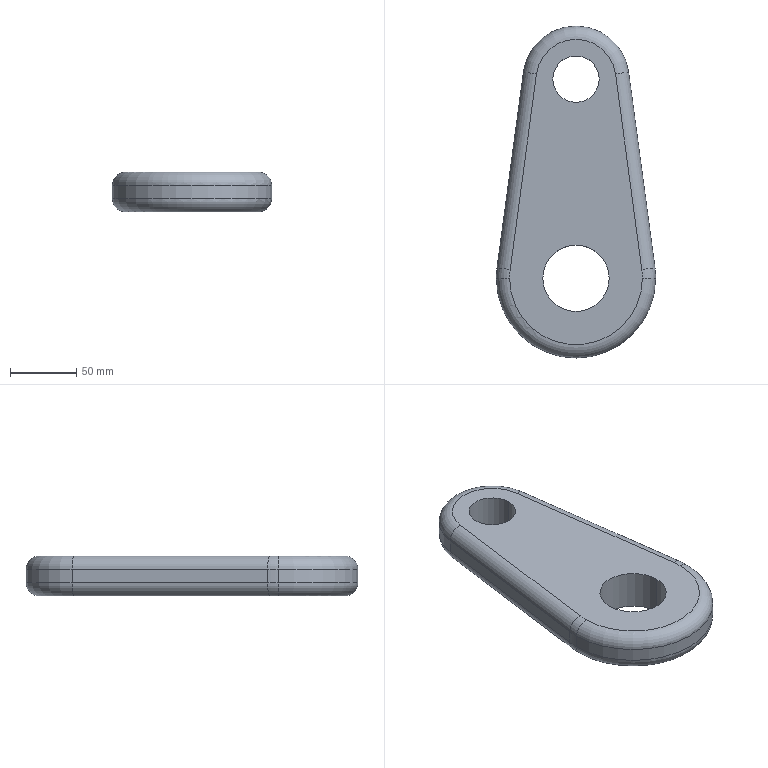Part | SolidWorks | features HoleWzd 2, Extrusion 1, Fillet 1 | 1 solid | 24 faces | box 120 x 250 x 30 mm | volume 585410 mm3 | cylinder 12 | torus 8 | plane 4 | commonest cylinder face diameters 20 x4 120 x3 35 x2 50 x2 80 x1
STEP:
#1=CARTESIAN_POINT('',(-50.,0.,0.));
#2=VERTEX_POINT('',#1);
#3=CARTESIAN_POINT('',(-49.554,6.667,0.));
#4=VERTEX_POINT('',#3);
#5=CARTESIAN_POINT('',(0.,0.,0.));
#6=DIRECTION('',(0.,0.,-1.));
#7=DIRECTION('',(1.,0.,0.));
#8=AXIS2_PLACEMENT_3D('',#5,#6,#7);
#9=CIRCLE('',#8,50.);
#10=EDGE_CURVE('',#2,#4,#9,.T.);
#11=ORIENTED_EDGE('',*,*,#10,.F.);
#12=CARTESIAN_POINT('',(-60.,0.,10.));
#13=VERTEX_POINT('',#12);
#14=CARTESIAN_POINT('',(-50.,0.,10.));
#15=DIRECTION('',(0.,1.,0.));
#16=DIRECTION('',(-1.,0.,0.));
#17=AXIS2_PLACEMENT_3D('',#14,#15,#16);
#18=CIRCLE('',#17,10.);
#19=EDGE_CURVE('',#2,#13,#18,.T.);
#20=ORIENTED_EDGE('',*,*,#19,.T.);
#21=CARTESIAN_POINT('',(-59.464,8.,10.));
#22=VERTEX_POINT('',#21);
#23=CARTESIAN_POINT('',(0.,0.,10.));
#24=DIRECTION('',(0.,0.,1.));
#25=DIRECTION('',(1.,0.,0.));
#26=AXIS2_PLACEMENT_3D('',#23,#24,#25);
#27=CIRCLE('',#26,60.);
#28=EDGE_CURVE('',#22,#13,#27,.T.);
#29=ORIENTED_EDGE('',*,*,#28,.F.);
#30=CARTESIAN_POINT('',(-49.554,6.667,10.));
#31=DIRECTION('',(-0.1333,-0.9911,0.));
#32=DIRECTION('',(0.9911,-0.1333,0.));
#33=AXIS2_PLACEMENT_3D('',#30,#31,#32);
#34=CIRCLE('',#33,10.);
#35=EDGE_CURVE('',#22,#4,#34,.T.);
#36=ORIENTED_EDGE('',*,*,#35,.T.);
#37=EDGE_LOOP('',(#11,#20,#29,#36));
#38=FACE_OUTER_BOUND('',#37,.T.);
#39=CARTESIAN_POINT('',(0.,0.,10.));
#40=DIRECTION('',(0.,0.,1.));
#41=DIRECTION('',(1.,0.,0.));
#42=AXIS2_PLACEMENT_3D('',#39,#40,#41);
#43=TOROIDAL_SURFACE('',#42,50.,10.);
#44=ADVANCED_FACE('',(#38),#43,.T.);
#45=ORIENTED_EDGE('',*,*,#19,.F.);
#46=CARTESIAN_POINT('',(50.,0.,0.));
#47=VERTEX_POINT('',#46);
#48=CARTESIAN_POINT('',(0.,0.,0.));
#49=DIRECTION('',(0.,0.,-1.));
#50=DIRECTION('',(1.,0.,0.));
#51=AXIS2_PLACEMENT_3D('',#48,#49,#50);
#52=CIRCLE('',#51,50.);
#53=EDGE_CURVE('',#47,#2,#52,.T.);
#54=ORIENTED_EDGE('',*,*,#53,.F.);
#55=CARTESIAN_POINT('',(60.,0.,10.));
#56=VERTEX_POINT('',#55);
#57=CARTESIAN_POINT('',(50.,0.,10.));
#58=DIRECTION('',(0.,-1.,0.));
#59=DIRECTION('',(0.,0.,-1.));
#60=AXIS2_PLACEMENT_3D('',#57,#58,#59);
#61=CIRCLE('',#60,10.);
#62=EDGE_CURVE('',#47,#56,#61,.T.);
#63=ORIENTED_EDGE('',*,*,#62,.T.);
#64=CARTESIAN_POINT('',(0.,0.,10.));
#65=DIRECTION('',(0.,0.,1.));
#66=DIRECTION('',(1.,0.,0.));
#67=AXIS2_PLACEMENT_3D('',#64,#65,#66);
#68=CIRCLE('',#67,60.);
#69=EDGE_CURVE('',#13,#56,#68,.T.);
#70=ORIENTED_EDGE('',*,*,#69,.F.);
#71=EDGE_LOOP('',(#45,#54,#63,#70));
#72=FACE_OUTER_BOUND('',#71,.T.);
#73=CARTESIAN_POINT('',(0.,0.,10.));
#74=DIRECTION('',(0.,0.,1.));
#75=DIRECTION('',(1.,0.,0.));
#76=AXIS2_PLACEMENT_3D('',#73,#74,#75);
#77=TOROIDAL_SURFACE('',#76,50.,10.);
#78=ADVANCED_FACE('',(#72),#77,.T.);
#79=CARTESIAN_POINT('',(-60.,0.,20.));
#80=VERTEX_POINT('',#79);
#81=CARTESIAN_POINT('',(-59.464,8.,20.));
#82=VERTEX_POINT('',#81);
#83=CARTESIAN_POINT('',(0.,0.,20.));
#84=DIRECTION('',(0.,0.,-1.));
#85=DIRECTION('',(1.,0.,0.));
#86=AXIS2_PLACEMENT_3D('',#83,#84,#85);
#87=CIRCLE('',#86,60.);
#88=EDGE_CURVE('',#80,#82,#87,.T.);
#89=ORIENTED_EDGE('',*,*,#88,.F.);
#90=CARTESIAN_POINT('',(-50.,0.,30.));
#91=VERTEX_POINT('',#90);
#92=CARTESIAN_POINT('',(-50.,0.,20.));
#93=DIRECTION('',(0.,1.,0.));
#94=DIRECTION('',(-1.,0.,0.));
#95=AXIS2_PLACEMENT_3D('',#92,#93,#94);
#96=CIRCLE('',#95,10.);
#97=EDGE_CURVE('',#80,#91,#96,.T.);
#98=ORIENTED_EDGE('',*,*,#97,.T.);
#99=CARTESIAN_POINT('',(-49.554,6.667,30.));
#100=VERTEX_POINT('',#99);
#101=CARTESIAN_POINT('',(0.,0.,30.));
#102=DIRECTION('',(0.,0.,1.));
#103=DIRECTION('',(1.,0.,0.));
#104=AXIS2_PLACEMENT_3D('',#101,#102,#103);
#105=CIRCLE('',#104,50.);
#106=EDGE_CURVE('',#100,#91,#105,.T.);
#107=ORIENTED_EDGE('',*,*,#106,.F.);
#108=CARTESIAN_POINT('',(-49.554,6.667,20.));
#109=DIRECTION('',(0.1333,0.9911,0.));
#110=DIRECTION('',(-0.9911,0.1333,0.));
#111=AXIS2_PLACEMENT_3D('',#108,#109,#110);
#112=CIRCLE('',#111,10.);
#113=EDGE_CURVE('',#82,#100,#112,.T.);
#114=ORIENTED_EDGE('',*,*,#113,.F.);
#115=EDGE_LOOP('',(#89,#98,#107,#114));
#116=FACE_OUTER_BOUND('',#115,.T.);
#117=CARTESIAN_POINT('',(0.,0.,20.));
#118=DIRECTION('',(0.,0.,1.));
#119=DIRECTION('',(1.,0.,0.));
#120=AXIS2_PLACEMENT_3D('',#117,#118,#119);
#121=TOROIDAL_SURFACE('',#120,50.,10.);
#122=ADVANCED_FACE('',(#116),#121,.T.);
#123=ORIENTED_EDGE('',*,*,#97,.F.);
#124=CARTESIAN_POINT('',(60.,0.,20.));
#125=VERTEX_POINT('',#124);
#126=CARTESIAN_POINT('',(0.,0.,20.));
#127=DIRECTION('',(0.,0.,-1.));
#128=DIRECTION('',(1.,0.,0.));
#129=AXIS2_PLACEMENT_3D('',#126,#127,#128);
#130=CIRCLE('',#129,60.);
#131=EDGE_CURVE('',#125,#80,#130,.T.);
#132=ORIENTED_EDGE('',*,*,#131,.F.);
#133=CARTESIAN_POINT('',(50.,0.,30.));
#134=VERTEX_POINT('',#133);
#135=CARTESIAN_POINT('',(50.,0.,20.));
#136=DIRECTION('',(0.,-1.,0.));
#137=DIRECTION('',(0.,0.,-1.));
#138=AXIS2_PLACEMENT_3D('',#135,#136,#137);
#139=CIRCLE('',#138,10.);
#140=EDGE_CURVE('',#125,#134,#139,.T.);
#141=ORIENTED_EDGE('',*,*,#140,.T.);
#142=CARTESIAN_POINT('',(0.,0.,30.));
#143=DIRECTION('',(0.,0.,1.));
#144=DIRECTION('',(1.,0.,0.));
#145=AXIS2_PLACEMENT_3D('',#142,#143,#144);
#146=CIRCLE('',#145,50.);
#147=EDGE_CURVE('',#91,#134,#146,.T.);
#148=ORIENTED_EDGE('',*,*,#147,.F.);
#149=EDGE_LOOP('',(#123,#132,#141,#148));
#150=FACE_OUTER_BOUND('',#149,.T.);
#151=CARTESIAN_POINT('',(0.,0.,20.));
#152=DIRECTION('',(0.,0.,1.));
#153=DIRECTION('',(1.,0.,0.));
#154=AXIS2_PLACEMENT_3D('',#151,#152,#153);
#155=TOROIDAL_SURFACE('',#154,50.,10.);
#156=ADVANCED_FACE('',(#150),#155,.T.);
#157=CARTESIAN_POINT('',(25.,0.,30.));
#158=VERTEX_POINT('',#157);
#159=CARTESIAN_POINT('',(-25.,0.,30.));
#160=VERTEX_POINT('',#159);
#161=CARTESIAN_POINT('',(0.,0.,30.));
#162=DIRECTION('',(0.,0.,-1.));
#163=DIRECTION('',(-1.,0.,0.));
#164=AXIS2_PLACEMENT_3D('',#161,#162,#163);
#165=CIRCLE('',#164,25.);
#166=EDGE_CURVE('',#158,#160,#165,.T.);
#167=ORIENTED_EDGE('',*,*,#166,.F.);
#168=CARTESIAN_POINT('',(25.,0.,0.));
#169=VERTEX_POINT('',#168);
#170=CARTESIAN_POINT('',(25.,0.,0.));
#171=DIRECTION('',(0.,0.,-1.));
#172=VECTOR('',#171,1000.);
#173=LINE('',#170,#172);
#174=EDGE_CURVE('',#158,#169,#173,.T.);
#175=ORIENTED_EDGE('',*,*,#174,.T.);
#176=CARTESIAN_POINT('',(-25.,0.,0.));
#177=VERTEX_POINT('',#176);
#178=CARTESIAN_POINT('',(0.,0.,0.));
#179=DIRECTION('',(0.,0.,-1.));
#180=DIRECTION('',(-1.,0.,0.));
#181=AXIS2_PLACEMENT_3D('',#178,#179,#180);
#182=CIRCLE('',#181,25.);
#183=EDGE_CURVE('',#169,#177,#182,.T.);
#184=ORIENTED_EDGE('',*,*,#183,.T.);
#185=CARTESIAN_POINT('',(-25.,0.,0.));
#186=DIRECTION('',(0.,0.,-1.));
#187=VECTOR('',#186,1000.);
#188=LINE('',#185,#187);
#189=EDGE_CURVE('',#160,#177,#188,.T.);
#190=ORIENTED_EDGE('',*,*,#189,.F.);
#191=EDGE_LOOP('',(#167,#175,#184,#190));
#192=FACE_OUTER_BOUND('',#191,.T.);
#193=CARTESIAN_POINT('',(0.,0.,0.));
#194=DIRECTION('',(0.,0.,-1.));
#195=DIRECTION('',(-1.,0.,0.));
#196=AXIS2_PLACEMENT_3D('',#193,#194,#195);
#197=CYLINDRICAL_SURFACE('',#196,25.);
#198=ADVANCED_FACE('',(#192),#197,.F.);
#199=CARTESIAN_POINT('',(17.5,150.,30.));
#200=VERTEX_POINT('',#199);
#201=CARTESIAN_POINT('',(-17.5,150.,30.));
#202=VERTEX_POINT('',#201);
#203=CARTESIAN_POINT('',(0.,150.,30.));
#204=DIRECTION('',(0.,0.,-1.));
#205=DIRECTION('',(-1.,0.,0.));
#206=AXIS2_PLACEMENT_3D('',#203,#204,#205);
#207=CIRCLE('',#206,17.5);
#208=EDGE_CURVE('',#200,#202,#207,.T.);
#209=ORIENTED_EDGE('',*,*,#208,.F.);
#210=CARTESIAN_POINT('',(17.5,150.,0.));
#211=VERTEX_POINT('',#210);
#212=CARTESIAN_POINT('',(17.5,150.,0.));
#213=DIRECTION('',(0.,0.,-1.));
#214=VECTOR('',#213,1000.);
#215=LINE('',#212,#214);
#216=EDGE_CURVE('',#200,#211,#215,.T.);
#217=ORIENTED_EDGE('',*,*,#216,.T.);
#218=CARTESIAN_POINT('',(-17.5,150.,0.));
#219=VERTEX_POINT('',#218);
#220=CARTESIAN_POINT('',(0.,150.,0.));
#221=DIRECTION('',(0.,0.,-1.));
#222=DIRECTION('',(-1.,0.,0.));
#223=AXIS2_PLACEMENT_3D('',#220,#221,#222);
#224=CIRCLE('',#223,17.5);
#225=EDGE_CURVE('',#211,#219,#224,.T.);
#226=ORIENTED_EDGE('',*,*,#225,.T.);
#227=CARTESIAN_POINT('',(-17.5,150.,0.));
#228=DIRECTION('',(0.,0.,-1.));
#229=VECTOR('',#228,1000.);
#230=LINE('',#227,#229);
#231=EDGE_CURVE('',#202,#219,#230,.T.);
#232=ORIENTED_EDGE('',*,*,#231,.F.);
#233=EDGE_LOOP('',(#209,#217,#226,#232));
#234=FACE_OUTER_BOUND('',#233,.T.);
#235=CARTESIAN_POINT('',(0.,150.,0.));
#236=DIRECTION('',(0.,0.,-1.));
#237=DIRECTION('',(-1.,0.,0.));
#238=AXIS2_PLACEMENT_3D('',#235,#236,#237);
#239=CYLINDRICAL_SURFACE('',#238,17.5);
#240=ADVANCED_FACE('',(#234),#239,.F.);
#241=ORIENTED_EDGE('',*,*,#28,.T.);
#242=CARTESIAN_POINT('',(-60.,0.,0.));
#243=DIRECTION('',(0.,0.,1.));
#244=VECTOR('',#243,1000.);
#245=LINE('',#242,#244);
#246=EDGE_CURVE('',#13,#80,#245,.T.);
#247=ORIENTED_EDGE('',*,*,#246,.T.);
#248=ORIENTED_EDGE('',*,*,#88,.T.);
#249=CARTESIAN_POINT('',(-59.464,8.,0.));
#250=DIRECTION('',(0.,0.,1.));
#251=VECTOR('',#250,1000.);
#252=LINE('',#249,#251);
#253=EDGE_CURVE('',#22,#82,#252,.T.);
#254=ORIENTED_EDGE('',*,*,#253,.F.);
#255=EDGE_LOOP('',(#241,#247,#248,#254));
#256=FACE_OUTER_BOUND('',#255,.T.);
#257=CARTESIAN_POINT('',(0.,0.,0.));
#258=DIRECTION('',(0.,0.,1.));
#259=DIRECTION('',(1.,0.,0.));
#260=AXIS2_PLACEMENT_3D('',#257,#258,#259);
#261=CYLINDRICAL_SURFACE('',#260,60.);
#262=ADVANCED_FACE('',(#256),#261,.T.);
#263=ORIENTED_EDGE('',*,*,#246,.F.);
#264=ORIENTED_EDGE('',*,*,#69,.T.);
#265=CARTESIAN_POINT('',(60.,0.,0.));
#266=DIRECTION('',(0.,0.,1.));
#267=VECTOR('',#266,1000.);
#268=LINE('',#265,#267);
#269=EDGE_CURVE('',#56,#125,#268,.T.);
#270=ORIENTED_EDGE('',*,*,#269,.T.);
#271=ORIENTED_EDGE('',*,*,#131,.T.);
#272=EDGE_LOOP('',(#263,#264,#270,#271));
#273=FACE_OUTER_BOUND('',#272,.T.);
#274=CARTESIAN_POINT('',(0.,0.,0.));
#275=DIRECTION('',(0.,0.,1.));
#276=DIRECTION('',(1.,0.,0.));
#277=AXIS2_PLACEMENT_3D('',#274,#275,#276);
#278=CYLINDRICAL_SURFACE('',#277,60.);
#279=ADVANCED_FACE('',(#273),#278,.T.);
#280=ORIENTED_EDGE('',*,*,#269,.F.);
#281=CARTESIAN_POINT('',(59.464,8.,10.));
#282=VERTEX_POINT('',#281);
#283=CARTESIAN_POINT('',(0.,0.,10.));
#284=DIRECTION('',(0.,0.,1.));
#285=DIRECTION('',(1.,0.,0.));
#286=AXIS2_PLACEMENT_3D('',#283,#284,#285);
#287=CIRCLE('',#286,60.);
#288=EDGE_CURVE('',#56,#282,#287,.T.);
#289=ORIENTED_EDGE('',*,*,#288,.T.);
#290=CARTESIAN_POINT('',(59.464,8.,20.));
#291=VERTEX_POINT('',#290);
#292=CARTESIAN_POINT('',(59.464,8.,0.));
#293=DIRECTION('',(0.,0.,1.));
#294=VECTOR('',#293,1000.);
#295=LINE('',#292,#294);
#296=EDGE_CURVE('',#282,#291,#295,.T.);
#297=ORIENTED_EDGE('',*,*,#296,.T.);
#298=CARTESIAN_POINT('',(0.,0.,20.));
#299=DIRECTION('',(0.,0.,-1.));
#300=DIRECTION('',(1.,0.,0.));
#301=AXIS2_PLACEMENT_3D('',#298,#299,#300);
#302=CIRCLE('',#301,60.);
#303=EDGE_CURVE('',#291,#125,#302,.T.);
#304=ORIENTED_EDGE('',*,*,#303,.T.);
#305=EDGE_LOOP('',(#280,#289,#297,#304));
#306=FACE_OUTER_BOUND('',#305,.T.);
#307=CARTESIAN_POINT('',(0.,0.,0.));
#308=DIRECTION('',(0.,0.,1.));
#309=DIRECTION('',(1.,0.,0.));
#310=AXIS2_PLACEMENT_3D('',#307,#308,#309);
#311=CYLINDRICAL_SURFACE('',#310,60.);
#312=ADVANCED_FACE('',(#306),#311,.T.);
#313=ORIENTED_EDGE('',*,*,#253,.T.);
#314=CARTESIAN_POINT('',(-39.643,155.333,20.));
#315=VERTEX_POINT('',#314);
#316=CARTESIAN_POINT('',(-39.643,155.333,20.));
#317=DIRECTION('',(0.1333,0.9911,0.));
#318=VECTOR('',#317,1000.);
#319=LINE('',#316,#318);
#320=EDGE_CURVE('',#82,#315,#319,.T.);
#321=ORIENTED_EDGE('',*,*,#320,.T.);
#322=CARTESIAN_POINT('',(-39.643,155.333,10.));
#323=VERTEX_POINT('',#322);
#324=CARTESIAN_POINT('',(-39.643,155.333,0.));
#325=DIRECTION('',(0.,0.,1.));
#326=VECTOR('',#325,1000.);
#327=LINE('',#324,#326);
#328=EDGE_CURVE('',#323,#315,#327,.T.);
#329=ORIENTED_EDGE('',*,*,#328,.F.);
#330=CARTESIAN_POINT('',(-59.464,8.,10.));
#331=DIRECTION('',(-0.1333,-0.9911,0.));
#332=VECTOR('',#331,1000.);
#333=LINE('',#330,#332);
#334=EDGE_CURVE('',#323,#22,#333,.T.);
#335=ORIENTED_EDGE('',*,*,#334,.T.);
#336=EDGE_LOOP('',(#313,#321,#329,#335));
#337=FACE_OUTER_BOUND('',#336,.T.);
#338=CARTESIAN_POINT('',(-39.643,155.333,0.));
#339=DIRECTION('',(-0.9911,0.1333,0.));
#340=DIRECTION('',(-0.1333,-0.9911,0.));
#341=AXIS2_PLACEMENT_3D('',#338,#339,#340);
#342=PLANE('',#341);
#343=ADVANCED_FACE('',(#337),#342,.T.);
#344=ORIENTED_EDGE('',*,*,#328,.T.);
#345=CARTESIAN_POINT('',(39.643,155.333,20.));
#346=VERTEX_POINT('',#345);
#347=CARTESIAN_POINT('',(0.,150.,20.));
#348=DIRECTION('',(0.,0.,-1.));
#349=DIRECTION('',(1.,0.,0.));
#350=AXIS2_PLACEMENT_3D('',#347,#348,#349);
#351=CIRCLE('',#350,40.);
#352=EDGE_CURVE('',#315,#346,#351,.T.);
#353=ORIENTED_EDGE('',*,*,#352,.T.);
#354=CARTESIAN_POINT('',(39.643,155.333,10.));
#355=VERTEX_POINT('',#354);
#356=CARTESIAN_POINT('',(39.643,155.333,0.));
#357=DIRECTION('',(0.,0.,1.));
#358=VECTOR('',#357,1000.);
#359=LINE('',#356,#358);
#360=EDGE_CURVE('',#355,#346,#359,.T.);
#361=ORIENTED_EDGE('',*,*,#360,.F.);
#362=CARTESIAN_POINT('',(0.,150.,10.));
#363=DIRECTION('',(0.,0.,1.));
#364=DIRECTION('',(1.,0.,0.));
#365=AXIS2_PLACEMENT_3D('',#362,#363,#364);
#366=CIRCLE('',#365,40.);
#367=EDGE_CURVE('',#355,#323,#366,.T.);
#368=ORIENTED_EDGE('',*,*,#367,.T.);
#369=EDGE_LOOP('',(#344,#353,#361,#368));
#370=FACE_OUTER_BOUND('',#369,.T.);
#371=CARTESIAN_POINT('',(0.,150.,0.));
#372=DIRECTION('',(0.,0.,1.));
#373=DIRECTION('',(1.,0.,0.));
#374=AXIS2_PLACEMENT_3D('',#371,#372,#373);
#375=CYLINDRICAL_SURFACE('',#374,40.);
#376=ADVANCED_FACE('',(#370),#375,.T.);
#377=ORIENTED_EDGE('',*,*,#360,.T.);
#378=CARTESIAN_POINT('',(59.464,8.,20.));
#379=DIRECTION('',(0.1333,-0.9911,0.));
#380=VECTOR('',#379,1000.);
#381=LINE('',#378,#380);
#382=EDGE_CURVE('',#346,#291,#381,.T.);
#383=ORIENTED_EDGE('',*,*,#382,.T.);
#384=ORIENTED_EDGE('',*,*,#296,.F.);
#385=CARTESIAN_POINT('',(39.643,155.333,10.));
#386=DIRECTION('',(-0.1333,0.9911,0.));
#387=VECTOR('',#386,1000.);
#388=LINE('',#385,#387);
#389=EDGE_CURVE('',#282,#355,#388,.T.);
#390=ORIENTED_EDGE('',*,*,#389,.T.);
#391=EDGE_LOOP('',(#377,#383,#384,#390));
#392=FACE_OUTER_BOUND('',#391,.T.);
#393=CARTESIAN_POINT('',(59.464,8.,0.));
#394=DIRECTION('',(0.9911,0.1333,0.));
#395=DIRECTION('',(-0.1333,0.9911,0.));
#396=AXIS2_PLACEMENT_3D('',#393,#394,#395);
#397=PLANE('',#396);
#398=ADVANCED_FACE('',(#392),#397,.T.);
#399=CARTESIAN_POINT('',(-29.732,154.,0.));
#400=VERTEX_POINT('',#399);
#401=CARTESIAN_POINT('',(29.732,154.,0.));
#402=VERTEX_POINT('',#401);
#403=CARTESIAN_POINT('',(0.,150.,0.));
#404=DIRECTION('',(0.,0.,-1.));
#405=DIRECTION('',(1.,0.,0.));
#406=AXIS2_PLACEMENT_3D('',#403,#404,#405);
#407=CIRCLE('',#406,30.);
#408=EDGE_CURVE('',#400,#402,#407,.T.);
#409=ORIENTED_EDGE('',*,*,#408,.T.);
#410=CARTESIAN_POINT('',(49.554,6.667,0.));
#411=VERTEX_POINT('',#410);
#412=CARTESIAN_POINT('',(49.554,6.667,0.));
#413=DIRECTION('',(0.1333,-0.9911,0.));
#414=VECTOR('',#413,1000.);
#415=LINE('',#412,#414);
#416=EDGE_CURVE('',#402,#411,#415,.T.);
#417=ORIENTED_EDGE('',*,*,#416,.T.);
#418=CARTESIAN_POINT('',(0.,0.,0.));
#419=DIRECTION('',(0.,0.,-1.));
#420=DIRECTION('',(1.,0.,0.));
#421=AXIS2_PLACEMENT_3D('',#418,#419,#420);
#422=CIRCLE('',#421,50.);
#423=EDGE_CURVE('',#411,#47,#422,.T.);
#424=ORIENTED_EDGE('',*,*,#423,.T.);
#425=ORIENTED_EDGE('',*,*,#53,.T.);
#426=ORIENTED_EDGE('',*,*,#10,.T.);
#427=CARTESIAN_POINT('',(-29.732,154.,0.));
#428=DIRECTION('',(0.1333,0.9911,0.));
#429=VECTOR('',#428,1000.);
#430=LINE('',#427,#429);
#431=EDGE_CURVE('',#4,#400,#430,.T.);
#432=ORIENTED_EDGE('',*,*,#431,.T.);
#433=EDGE_LOOP('',(#409,#417,#424,#425,#426,#432));
#434=FACE_OUTER_BOUND('',#433,.T.);
#435=CARTESIAN_POINT('',(0.,0.,0.));
#436=DIRECTION('',(0.,0.,-1.));
#437=DIRECTION('',(-1.,0.,0.));
#438=AXIS2_PLACEMENT_3D('',#435,#436,#437);
#439=CIRCLE('',#438,25.);
#440=EDGE_CURVE('',#177,#169,#439,.T.);
#441=ORIENTED_EDGE('',*,*,#440,.F.);
#442=ORIENTED_EDGE('',*,*,#183,.F.);
#443=EDGE_LOOP('',(#441,#442));
#444=FACE_BOUND('',#443,.T.);
#445=CARTESIAN_POINT('',(0.,150.,0.));
#446=DIRECTION('',(0.,0.,-1.));
#447=DIRECTION('',(-1.,0.,0.));
#448=AXIS2_PLACEMENT_3D('',#445,#446,#447);
#449=CIRCLE('',#448,17.5);
#450=EDGE_CURVE('',#219,#211,#449,.T.);
#451=ORIENTED_EDGE('',*,*,#450,.F.);
#452=ORIENTED_EDGE('',*,*,#225,.F.);
#453=EDGE_LOOP('',(#451,#452));
#454=FACE_BOUND('',#453,.T.);
#455=CARTESIAN_POINT('',(0.,0.,0.));
#456=DIRECTION('',(0.,0.,1.));
#457=DIRECTION('',(1.,0.,0.));
#458=AXIS2_PLACEMENT_3D('',#455,#456,#457);
#459=PLANE('',#458);
#460=ADVANCED_FACE('',(#434,#444,#454),#459,.F.);
#461=CARTESIAN_POINT('',(49.554,6.667,30.));
#462=VERTEX_POINT('',#461);
#463=CARTESIAN_POINT('',(29.732,154.,30.));
#464=VERTEX_POINT('',#463);
#465=CARTESIAN_POINT('',(49.554,6.667,30.));
#466=DIRECTION('',(-0.1333,0.9911,0.));
#467=VECTOR('',#466,1000.);
#468=LINE('',#465,#467);
#469=EDGE_CURVE('',#462,#464,#468,.T.);
#470=ORIENTED_EDGE('',*,*,#469,.T.);
#471=CARTESIAN_POINT('',(-29.732,154.,30.));
#472=VERTEX_POINT('',#471);
#473=CARTESIAN_POINT('',(0.,150.,30.));
#474=DIRECTION('',(0.,0.,1.));
#475=DIRECTION('',(1.,0.,0.));
#476=AXIS2_PLACEMENT_3D('',#473,#474,#475);
#477=CIRCLE('',#476,30.);
#478=EDGE_CURVE('',#464,#472,#477,.T.);
#479=ORIENTED_EDGE('',*,*,#478,.T.);
#480=CARTESIAN_POINT('',(-49.554,6.667,30.));
#481=DIRECTION('',(-0.1333,-0.9911,0.));
#482=VECTOR('',#481,1000.);
#483=LINE('',#480,#482);
#484=EDGE_CURVE('',#472,#100,#483,.T.);
#485=ORIENTED_EDGE('',*,*,#484,.T.);
#486=ORIENTED_EDGE('',*,*,#106,.T.);
#487=ORIENTED_EDGE('',*,*,#147,.T.);
#488=CARTESIAN_POINT('',(0.,0.,30.));
#489=DIRECTION('',(0.,0.,1.));
#490=DIRECTION('',(1.,0.,0.));
#491=AXIS2_PLACEMENT_3D('',#488,#489,#490);
#492=CIRCLE('',#491,50.);
#493=EDGE_CURVE('',#134,#462,#492,.T.);
#494=ORIENTED_EDGE('',*,*,#493,.T.);
#495=EDGE_LOOP('',(#470,#479,#485,#486,#487,#494));
#496=FACE_OUTER_BOUND('',#495,.T.);
#497=CARTESIAN_POINT('',(0.,0.,30.));
#498=DIRECTION('',(0.,0.,-1.));
#499=DIRECTION('',(-1.,0.,0.));
#500=AXIS2_PLACEMENT_3D('',#497,#498,#499);
#501=CIRCLE('',#500,25.);
#502=EDGE_CURVE('',#160,#158,#501,.T.);
#503=ORIENTED_EDGE('',*,*,#502,.T.);
#504=ORIENTED_EDGE('',*,*,#166,.T.);
#505=EDGE_LOOP('',(#503,#504));
#506=FACE_BOUND('',#505,.T.);
#507=CARTESIAN_POINT('',(0.,150.,30.));
#508=DIRECTION('',(0.,0.,-1.));
#509=DIRECTION('',(-1.,0.,0.));
#510=AXIS2_PLACEMENT_3D('',#507,#508,#509);
#511=CIRCLE('',#510,17.5);
#512=EDGE_CURVE('',#202,#200,#511,.T.);
#513=ORIENTED_EDGE('',*,*,#512,.T.);
#514=ORIENTED_EDGE('',*,*,#208,.T.);
#515=EDGE_LOOP('',(#513,#514));
#516=FACE_BOUND('',#515,.T.);
#517=CARTESIAN_POINT('',(0.,0.,30.));
#518=DIRECTION('',(0.,0.,1.));
#519=DIRECTION('',(1.,0.,0.));
#520=AXIS2_PLACEMENT_3D('',#517,#518,#519);
#521=PLANE('',#520);
#522=ADVANCED_FACE('',(#496,#506,#516),#521,.T.);
#523=ORIENTED_EDGE('',*,*,#216,.F.);
#524=ORIENTED_EDGE('',*,*,#512,.F.);
#525=ORIENTED_EDGE('',*,*,#231,.T.);
#526=ORIENTED_EDGE('',*,*,#450,.T.);
#527=EDGE_LOOP('',(#523,#524,#525,#526));
#528=FACE_OUTER_BOUND('',#527,.T.);
#529=CARTESIAN_POINT('',(0.,150.,0.));
#530=DIRECTION('',(0.,0.,-1.));
#531=DIRECTION('',(-1.,0.,0.));
#532=AXIS2_PLACEMENT_3D('',#529,#530,#531);
#533=CYLINDRICAL_SURFACE('',#532,17.5);
#534=ADVANCED_FACE('',(#528),#533,.F.);
#535=ORIENTED_EDGE('',*,*,#174,.F.);
#536=ORIENTED_EDGE('',*,*,#502,.F.);
#537=ORIENTED_EDGE('',*,*,#189,.T.);
#538=ORIENTED_EDGE('',*,*,#440,.T.);
#539=EDGE_LOOP('',(#535,#536,#537,#538));
#540=FACE_OUTER_BOUND('',#539,.T.);
#541=CARTESIAN_POINT('',(0.,0.,0.));
#542=DIRECTION('',(0.,0.,-1.));
#543=DIRECTION('',(-1.,0.,0.));
#544=AXIS2_PLACEMENT_3D('',#541,#542,#543);
#545=CYLINDRICAL_SURFACE('',#544,25.);
#546=ADVANCED_FACE('',(#540),#545,.F.);
#547=ORIENTED_EDGE('',*,*,#140,.F.);
#548=ORIENTED_EDGE('',*,*,#303,.F.);
#549=CARTESIAN_POINT('',(49.554,6.667,20.));
#550=DIRECTION('',(-0.1333,0.9911,0.));
#551=DIRECTION('',(-0.9911,-0.1333,0.));
#552=AXIS2_PLACEMENT_3D('',#549,#550,#551);
#553=CIRCLE('',#552,10.);
#554=EDGE_CURVE('',#462,#291,#553,.T.);
#555=ORIENTED_EDGE('',*,*,#554,.F.);
#556=ORIENTED_EDGE('',*,*,#493,.F.);
#557=EDGE_LOOP('',(#547,#548,#555,#556));
#558=FACE_OUTER_BOUND('',#557,.T.);
#559=CARTESIAN_POINT('',(0.,0.,20.));
#560=DIRECTION('',(0.,0.,1.));
#561=DIRECTION('',(1.,0.,0.));
#562=AXIS2_PLACEMENT_3D('',#559,#560,#561);
#563=TOROIDAL_SURFACE('',#562,50.,10.);
#564=ADVANCED_FACE('',(#558),#563,.T.);
#565=ORIENTED_EDGE('',*,*,#554,.T.);
#566=ORIENTED_EDGE('',*,*,#382,.F.);
#567=CARTESIAN_POINT('',(29.732,154.,20.));
#568=DIRECTION('',(-0.1333,0.9911,0.));
#569=DIRECTION('',(-0.9911,-0.1333,0.));
#570=AXIS2_PLACEMENT_3D('',#567,#568,#569);
#571=CIRCLE('',#570,10.);
#572=EDGE_CURVE('',#464,#346,#571,.T.);
#573=ORIENTED_EDGE('',*,*,#572,.F.);
#574=ORIENTED_EDGE('',*,*,#469,.F.);
#575=EDGE_LOOP('',(#565,#566,#573,#574));
#576=FACE_OUTER_BOUND('',#575,.T.);
#577=CARTESIAN_POINT('',(49.554,6.667,20.));
#578=DIRECTION('',(-0.1333,0.9911,0.));
#579=DIRECTION('',(-0.9911,-0.1333,0.));
#580=AXIS2_PLACEMENT_3D('',#577,#578,#579);
#581=CYLINDRICAL_SURFACE('',#580,10.);
#582=ADVANCED_FACE('',(#576),#581,.T.);
#583=ORIENTED_EDGE('',*,*,#113,.T.);
#584=ORIENTED_EDGE('',*,*,#484,.F.);
#585=CARTESIAN_POINT('',(-29.732,154.,20.));
#586=DIRECTION('',(0.1333,0.9911,0.));
#587=DIRECTION('',(-0.9911,0.1333,0.));
#588=AXIS2_PLACEMENT_3D('',#585,#586,#587);
#589=CIRCLE('',#588,10.);
#590=EDGE_CURVE('',#315,#472,#589,.T.);
#591=ORIENTED_EDGE('',*,*,#590,.F.);
#592=ORIENTED_EDGE('',*,*,#320,.F.);
#593=EDGE_LOOP('',(#583,#584,#591,#592));
#594=FACE_OUTER_BOUND('',#593,.T.);
#595=CARTESIAN_POINT('',(-49.554,6.667,20.));
#596=DIRECTION('',(-0.1333,-0.9911,0.));
#597=DIRECTION('',(0.9911,-0.1333,0.));
#598=AXIS2_PLACEMENT_3D('',#595,#596,#597);
#599=CYLINDRICAL_SURFACE('',#598,10.);
#600=ADVANCED_FACE('',(#594),#599,.T.);
#601=ORIENTED_EDGE('',*,*,#572,.T.);
#602=ORIENTED_EDGE('',*,*,#352,.F.);
#603=ORIENTED_EDGE('',*,*,#590,.T.);
#604=ORIENTED_EDGE('',*,*,#478,.F.);
#605=EDGE_LOOP('',(#601,#602,#603,#604));
#606=FACE_OUTER_BOUND('',#605,.T.);
#607=CARTESIAN_POINT('',(0.,150.,20.));
#608=DIRECTION('',(0.,0.,1.));
#609=DIRECTION('',(1.,0.,0.));
#610=AXIS2_PLACEMENT_3D('',#607,#608,#609);
#611=TOROIDAL_SURFACE('',#610,30.,10.);
#612=ADVANCED_FACE('',(#606),#611,.T.);
#613=CARTESIAN_POINT('',(-29.732,154.,10.));
#614=DIRECTION('',(0.1333,0.9911,0.));
#615=DIRECTION('',(-0.9911,0.1333,0.));
#616=AXIS2_PLACEMENT_3D('',#613,#614,#615);
#617=CIRCLE('',#616,10.);
#618=EDGE_CURVE('',#400,#323,#617,.T.);
#619=ORIENTED_EDGE('',*,*,#618,.F.);
#620=ORIENTED_EDGE('',*,*,#431,.F.);
#621=ORIENTED_EDGE('',*,*,#35,.F.);
#622=ORIENTED_EDGE('',*,*,#334,.F.);
#623=EDGE_LOOP('',(#619,#620,#621,#622));
#624=FACE_OUTER_BOUND('',#623,.T.);
#625=CARTESIAN_POINT('',(-29.732,154.,10.));
#626=DIRECTION('',(0.1333,0.9911,0.));
#627=DIRECTION('',(-0.9911,0.1333,0.));
#628=AXIS2_PLACEMENT_3D('',#625,#626,#627);
#629=CYLINDRICAL_SURFACE('',#628,10.);
#630=ADVANCED_FACE('',(#624),#629,.T.);
#631=ORIENTED_EDGE('',*,*,#62,.F.);
#632=ORIENTED_EDGE('',*,*,#423,.F.);
#633=CARTESIAN_POINT('',(49.554,6.667,10.));
#634=DIRECTION('',(-0.1333,0.9911,0.));
#635=DIRECTION('',(-0.9911,-0.1333,0.));
#636=AXIS2_PLACEMENT_3D('',#633,#634,#635);
#637=CIRCLE('',#636,10.);
#638=EDGE_CURVE('',#282,#411,#637,.T.);
#639=ORIENTED_EDGE('',*,*,#638,.F.);
#640=ORIENTED_EDGE('',*,*,#288,.F.);
#641=EDGE_LOOP('',(#631,#632,#639,#640));
#642=FACE_OUTER_BOUND('',#641,.T.);
#643=CARTESIAN_POINT('',(0.,0.,10.));
#644=DIRECTION('',(0.,0.,1.));
#645=DIRECTION('',(1.,0.,0.));
#646=AXIS2_PLACEMENT_3D('',#643,#644,#645);
#647=TOROIDAL_SURFACE('',#646,50.,10.);
#648=ADVANCED_FACE('',(#642),#647,.T.);
#649=ORIENTED_EDGE('',*,*,#618,.T.);
#650=ORIENTED_EDGE('',*,*,#367,.F.);
#651=CARTESIAN_POINT('',(29.732,154.,10.));
#652=DIRECTION('',(0.1333,-0.9911,0.));
#653=DIRECTION('',(0.9911,0.1333,0.));
#654=AXIS2_PLACEMENT_3D('',#651,#652,#653);
#655=CIRCLE('',#654,10.);
#656=EDGE_CURVE('',#402,#355,#655,.T.);
#657=ORIENTED_EDGE('',*,*,#656,.F.);
#658=ORIENTED_EDGE('',*,*,#408,.F.);
#659=EDGE_LOOP('',(#649,#650,#657,#658));
#660=FACE_OUTER_BOUND('',#659,.T.);
#661=CARTESIAN_POINT('',(0.,150.,10.));
#662=DIRECTION('',(0.,0.,1.));
#663=DIRECTION('',(1.,0.,0.));
#664=AXIS2_PLACEMENT_3D('',#661,#662,#663);
#665=TOROIDAL_SURFACE('',#664,30.,10.);
#666=ADVANCED_FACE('',(#660),#665,.T.);
#667=ORIENTED_EDGE('',*,*,#638,.T.);
#668=ORIENTED_EDGE('',*,*,#416,.F.);
#669=ORIENTED_EDGE('',*,*,#656,.T.);
#670=ORIENTED_EDGE('',*,*,#389,.F.);
#671=EDGE_LOOP('',(#667,#668,#669,#670));
#672=FACE_OUTER_BOUND('',#671,.T.);
#673=CARTESIAN_POINT('',(49.554,6.667,10.));
#674=DIRECTION('',(0.1333,-0.9911,0.));
#675=DIRECTION('',(0.9911,0.1333,0.));
#676=AXIS2_PLACEMENT_3D('',#673,#674,#675);
#677=CYLINDRICAL_SURFACE('',#676,10.);
#678=ADVANCED_FACE('',(#672),#677,.T.);
#679=CLOSED_SHELL('',(#44,#78,#122,#156,#198,#240,#262,#279,#312,#343,#376,#398,#460,#522,#534,#546,#564,#582,#600,#612,#630,#648,#666,#678));
#680=MANIFOLD_SOLID_BREP('',#679);
#681=CARTESIAN_POINT('',(0.,0.,0.));
#682=DIRECTION('',(0.,0.,1.));
#683=DIRECTION('',(1.,0.,0.));
#684=AXIS2_PLACEMENT_3D('',#681,#682,#683);
#685=(LENGTH_UNIT()NAMED_UNIT(*)SI_UNIT(.MILLI.,.METRE.));
#686=UNCERTAINTY_MEASURE_WITH_UNIT(LENGTH_MEASURE(0.00001),#685,'','');
#687=(NAMED_UNIT(*)PLANE_ANGLE_UNIT()SI_UNIT($,.RADIAN.));
#688=(NAMED_UNIT(*)SI_UNIT($,.STERADIAN.)SOLID_ANGLE_UNIT());
#689=(GEOMETRIC_REPRESENTATION_CONTEXT(3)GLOBAL_UNCERTAINTY_ASSIGNED_CONTEXT((#686))GLOBAL_UNIT_ASSIGNED_CONTEXT((#685,#687,#688))REPRESENTATION_CONTEXT('',''));
#690=ADVANCED_BREP_SHAPE_REPRESENTATION('',(#680,#684),#689);